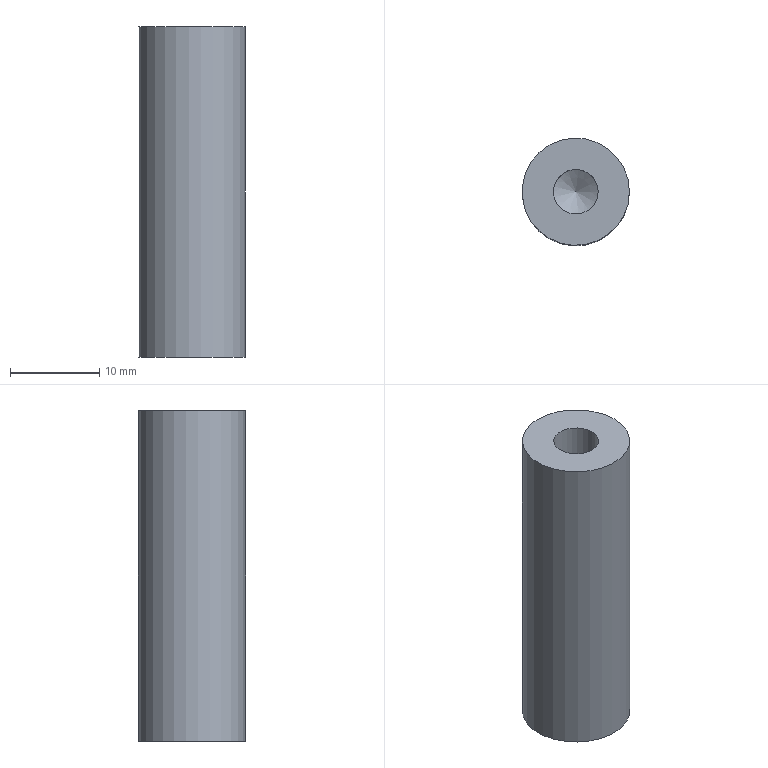Part | NX | features BREP 1 | 1 solid | 7 faces | box 12 x 12 x 37 mm | volume 3654 mm3 | cylinder 3 | cone 2 | plane 2 | commonest cylinder face diameters 5 x2 12 x1
STEP:
#1=CARTESIAN_POINT('',(2.5,0.,37.));
#2=VERTEX_POINT('',#1);
#3=CARTESIAN_POINT('',(0.,0.,37.));
#4=DIRECTION('',(0.,0.,1.));
#5=DIRECTION('',(1.,0.,0.));
#6=AXIS2_PLACEMENT_3D('',#3,#4,#5);
#7=CIRCLE('',#6,2.5);
#8=EDGE_CURVE('',#2,#2,#7,.T.);
#9=ORIENTED_EDGE('',*,*,#8,.T.);
#10=EDGE_LOOP('',(#9));
#11=FACE_BOUND('',#10,.T.);
#12=CARTESIAN_POINT('',(2.5,0.,24.));
#13=VERTEX_POINT('',#12);
#14=CARTESIAN_POINT('',(0.,0.,24.));
#15=DIRECTION('',(0.,0.,1.));
#16=DIRECTION('',(1.,0.,0.));
#17=AXIS2_PLACEMENT_3D('',#14,#15,#16);
#18=CIRCLE('',#17,2.5);
#19=EDGE_CURVE('',#13,#13,#18,.T.);
#20=ORIENTED_EDGE('',*,*,#19,.F.);
#21=EDGE_LOOP('',(#20));
#22=FACE_BOUND('',#21,.T.);
#23=CARTESIAN_POINT('',(0.,0.,37.));
#24=DIRECTION('',(0.,0.,1.));
#25=DIRECTION('',(1.,0.,0.));
#26=AXIS2_PLACEMENT_3D('',#23,#24,#25);
#27=CYLINDRICAL_SURFACE('',#26,2.5);
#28=ADVANCED_FACE('',(#11,#22),#27,.F.);
#29=ORIENTED_EDGE('',*,*,#19,.T.);
#30=EDGE_LOOP('',(#29));
#31=FACE_BOUND('',#30,.T.);
#32=CARTESIAN_POINT('',(0.,0.,22.498));
#33=VERTEX_POINT('',#32);
#34=VERTEX_LOOP('',#33);
#35=FACE_BOUND('',#34,.T.);
#36=CARTESIAN_POINT('',(0.,0.,24.));
#37=DIRECTION('',(0.,0.,1.));
#38=DIRECTION('',(1.,0.,0.));
#39=AXIS2_PLACEMENT_3D('',#36,#37,#38);
#40=CONICAL_SURFACE('',#39,2.5,1.03);
#41=ADVANCED_FACE('',(#31,#35),#40,.F.);
#42=CARTESIAN_POINT('',(-2.5,0.,0.));
#43=VERTEX_POINT('',#42);
#44=CARTESIAN_POINT('',(0.,0.,0.));
#45=DIRECTION('',(0.,0.,-1.));
#46=DIRECTION('',(-1.,0.,0.));
#47=AXIS2_PLACEMENT_3D('',#44,#45,#46);
#48=CIRCLE('',#47,2.5);
#49=EDGE_CURVE('',#43,#43,#48,.T.);
#50=ORIENTED_EDGE('',*,*,#49,.T.);
#51=EDGE_LOOP('',(#50));
#52=FACE_BOUND('',#51,.T.);
#53=CARTESIAN_POINT('',(-2.5,0.,13.));
#54=VERTEX_POINT('',#53);
#55=CARTESIAN_POINT('',(0.,0.,13.));
#56=DIRECTION('',(0.,0.,-1.));
#57=DIRECTION('',(-1.,0.,0.));
#58=AXIS2_PLACEMENT_3D('',#55,#56,#57);
#59=CIRCLE('',#58,2.5);
#60=EDGE_CURVE('',#54,#54,#59,.T.);
#61=ORIENTED_EDGE('',*,*,#60,.F.);
#62=EDGE_LOOP('',(#61));
#63=FACE_BOUND('',#62,.T.);
#64=CARTESIAN_POINT('',(0.,0.,0.));
#65=DIRECTION('',(0.,0.,-1.));
#66=DIRECTION('',(-1.,0.,0.));
#67=AXIS2_PLACEMENT_3D('',#64,#65,#66);
#68=CYLINDRICAL_SURFACE('',#67,2.5);
#69=ADVANCED_FACE('',(#52,#63),#68,.F.);
#70=ORIENTED_EDGE('',*,*,#60,.T.);
#71=EDGE_LOOP('',(#70));
#72=FACE_BOUND('',#71,.T.);
#73=CARTESIAN_POINT('',(0.,0.,14.502));
#74=VERTEX_POINT('',#73);
#75=VERTEX_LOOP('',#74);
#76=FACE_BOUND('',#75,.T.);
#77=CARTESIAN_POINT('',(0.,0.,13.));
#78=DIRECTION('',(0.,0.,-1.));
#79=DIRECTION('',(-1.,0.,0.));
#80=AXIS2_PLACEMENT_3D('',#77,#78,#79);
#81=CONICAL_SURFACE('',#80,2.5,1.03);
#82=ADVANCED_FACE('',(#72,#76),#81,.F.);
#83=CARTESIAN_POINT('',(6.,0.,0.));
#84=VERTEX_POINT('',#83);
#85=CARTESIAN_POINT('',(0.,0.,0.));
#86=DIRECTION('',(0.,0.,1.));
#87=DIRECTION('',(1.,0.,0.));
#88=AXIS2_PLACEMENT_3D('',#85,#86,#87);
#89=CIRCLE('',#88,6.);
#90=EDGE_CURVE('',#84,#84,#89,.T.);
#91=ORIENTED_EDGE('',*,*,#90,.T.);
#92=EDGE_LOOP('',(#91));
#93=FACE_BOUND('',#92,.T.);
#94=CARTESIAN_POINT('',(6.,0.,37.));
#95=VERTEX_POINT('',#94);
#96=CARTESIAN_POINT('',(0.,0.,37.));
#97=DIRECTION('',(0.,0.,1.));
#98=DIRECTION('',(1.,0.,0.));
#99=AXIS2_PLACEMENT_3D('',#96,#97,#98);
#100=CIRCLE('',#99,6.);
#101=EDGE_CURVE('',#95,#95,#100,.T.);
#102=ORIENTED_EDGE('',*,*,#101,.F.);
#103=EDGE_LOOP('',(#102));
#104=FACE_BOUND('',#103,.T.);
#105=CARTESIAN_POINT('',(0.,0.,37.));
#106=DIRECTION('',(0.,0.,-1.));
#107=DIRECTION('',(-1.,0.,0.));
#108=AXIS2_PLACEMENT_3D('',#105,#106,#107);
#109=CYLINDRICAL_SURFACE('',#108,6.);
#110=ADVANCED_FACE('',(#93,#104),#109,.T.);
#111=ORIENTED_EDGE('',*,*,#8,.F.);
#112=EDGE_LOOP('',(#111));
#113=FACE_BOUND('',#112,.T.);
#114=ORIENTED_EDGE('',*,*,#101,.T.);
#115=EDGE_LOOP('',(#114));
#116=FACE_BOUND('',#115,.T.);
#117=CARTESIAN_POINT('',(0.,0.,37.));
#118=DIRECTION('',(0.,0.,1.));
#119=DIRECTION('',(1.,0.,0.));
#120=AXIS2_PLACEMENT_3D('',#117,#118,#119);
#121=PLANE('',#120);
#122=ADVANCED_FACE('',(#113,#116),#121,.T.);
#123=ORIENTED_EDGE('',*,*,#49,.F.);
#124=EDGE_LOOP('',(#123));
#125=FACE_BOUND('',#124,.T.);
#126=ORIENTED_EDGE('',*,*,#90,.F.);
#127=EDGE_LOOP('',(#126));
#128=FACE_BOUND('',#127,.T.);
#129=CARTESIAN_POINT('',(0.,0.,0.));
#130=DIRECTION('',(0.,0.,1.));
#131=DIRECTION('',(1.,0.,0.));
#132=AXIS2_PLACEMENT_3D('',#129,#130,#131);
#133=PLANE('',#132);
#134=ADVANCED_FACE('',(#125,#128),#133,.F.);
#135=CLOSED_SHELL('',(#28,#41,#69,#82,#110,#122,#134));
#136=MANIFOLD_SOLID_BREP('',#135);
#137=(LENGTH_UNIT()NAMED_UNIT(*)SI_UNIT(.MILLI.,.METRE.));
#138=UNCERTAINTY_MEASURE_WITH_UNIT(LENGTH_MEASURE(0.00001),#137,'','');
#139=(NAMED_UNIT(*)PLANE_ANGLE_UNIT()SI_UNIT($,.RADIAN.));
#140=(NAMED_UNIT(*)SI_UNIT($,.STERADIAN.)SOLID_ANGLE_UNIT());
#141=(GEOMETRIC_REPRESENTATION_CONTEXT(3)GLOBAL_UNCERTAINTY_ASSIGNED_CONTEXT((#138))GLOBAL_UNIT_ASSIGNED_CONTEXT((#137,#139,#140))REPRESENTATION_CONTEXT('',''));
#142=ADVANCED_BREP_SHAPE_REPRESENTATION('',(#136),#141);